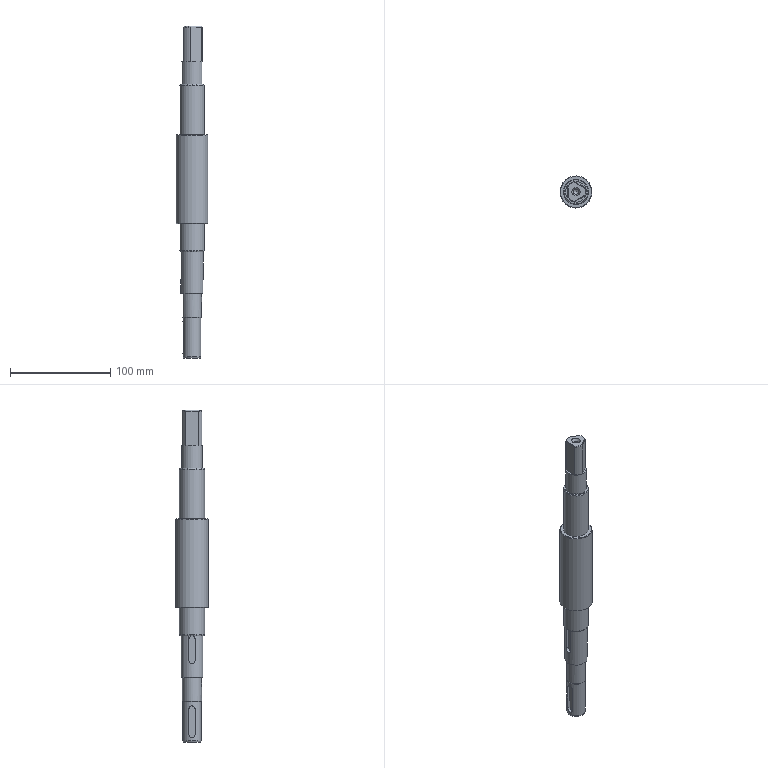NC program | NX | posted with a generic post | part box 32 x 32 x 331.3 mm
Lines 26 to 959 of 3379:
(ZLEVEL_PROFILE , TOOL : D12)
N44 T12 M6
N46 G54
N48 G17 G0 G90 X2.858 Y-14.112 B0. C0. S3000 M3
N50 G43 Z30. H12
N52 Z3.
N54 G94 G1 X1.878 Y-14.678 Z2.97 F1000.
N56 X1.831 Y-14.699 Z2.969
N58 X1.427 Y-14.934 Z2.957
N60 X1.001 Y-15.192 Z2.944
N62 X0.023 Y-15.693 Z2.915
N64 X-1.127 Y-16.017 Z2.884
N66 X-2.318 Y-16.109 Z2.852
N68 X-2.915 Y-16.036 Z2.837
N70 X-3.072 Y-16.017 Z2.833
N72 X-5.029 Y-15.657 Z2.78
N74 X-7.08 Y-14.962 Z2.724
N76 X-7.355 Y-14.847 Z2.716
N78 X-8.788 Y-14.141 Z2.674
N80 X-8.843 Y-14.118 Z2.672
N82 X-9.05 Y-14.001 Z2.666
N84 X-10.687 Y-12.925 Z2.615
N86 X-10.869 Y-12.784 Z2.609
N88 X-11.079 Y-12.619 Z2.602
N90 X-12.428 Y-11.41 Z2.555
N92 X-12.651 Y-11.181 Z2.546
N94 X-13.853 Y-9.785 Z2.498
N96 X-14.227 Y-9.302 Z2.482
N98 X-14.846 Y-8.002 Z2.444
N100 X-15.15 Y-6.595 Z2.407
N102 Y-5.985 Z2.391
N104 Y5.985 Z2.077
N106 X-15.152 Y6.593 Z2.061
N108 X-14.802 Y8.127 Z2.02
N110 X-14.077 Y9.524 Z1.979
N112 X-13.683 Y9.987 Z1.963
N114 X-12.756 Y11.07 Z1.926
N116 X-12.545 Y11.293 Z1.917
N118 X-11.116 Y12.59 Z1.867
N120 X-10.866 Y12.786 Z1.859
N122 X-9.251 Y13.882 Z1.808
N124 X-8.895 Y14.089 Z1.797
N126 X-7.378 Y14.834 Z1.752
N128 X-7.006 Y14.992 Z1.742
N130 X-5.308 Y15.565 Z1.695
N132 X-4.231 Y15.83 Z1.666
N134 X-3.137 Y16.009 Z1.637
N136 X-2.539 Y16.103 Z1.621
N138 X-1.05 Y16.006 Z1.582
N140 X0.371 Y15.552 Z1.543
N142 X0.894 Y15.246 Z1.527
N144 X10.315 Y9.803 Z1.242
N146 X11.822 Y8.929 Z1.197
N148 X12.828 Y8.019 Z1.161
N150 X13.61 Y6.909 Z1.125
N152 X13.848 Y6.352 Z1.11
N154 X14.242 Y5.407 Z1.083
N156 X14.801 Y3.449 Z1.029
N158 X14.965 Y2.438 Z1.003
N160 X15.109 Y1.428 Z0.976
N162 X15.148 Y-0.892 Z0.915
N164 X15.037 Y-1.907 Z0.888
N166 X14.905 Y-2.923 Z0.862
N168 X14.326 Y-5.155 Z0.801
N170 X13.948 Y-6.106 Z0.774
N172 X13.724 Y-6.681 Z0.758
N174 X12.892 Y-7.93 Z0.719
N176 X11.79 Y-8.95 Z0.68
N178 X11.258 Y-9.262 Z0.663
N180 X1.878 Y-14.678 Z0.38
N182 X1.831 Y-14.699 Z0.378
N184 X1.427 Y-14.934 Z0.366
N186 X1.001 Y-15.192 Z0.353
N188 X0.023 Y-15.693 Z0.324
N190 X-1.127 Y-16.017 Z0.293
N192 X-2.318 Y-16.109 Z0.262
N194 X-2.915 Y-16.036 Z0.246
N196 X-3.072 Y-16.017 Z0.242
N198 X-5.029 Y-15.657 Z0.19
N200 X-7.08 Y-14.962 Z0.133
N202 X-7.355 Y-14.847 Z0.125
N204 X-8.788 Y-14.141 Z0.084
N206 X-8.843 Y-14.118 Z0.082
N208 X-9.05 Y-14.001 Z0.076
N210 X-10.687 Y-12.925 Z0.024
N212 X-10.869 Y-12.784 Z0.018
N214 X-11.079 Y-12.619 Z0.011
N216 X-12.428 Y-11.41 Z-0.036
N218 X-12.651 Y-11.181 Z-0.044
N220 X-13.853 Y-9.785 Z-0.093
N222 X-14.227 Y-9.302 Z-0.109
N224 X-14.846 Y-8.002 Z-0.146
N226 X-15.15 Y-6.595 Z-0.184
N228 Y-5.985 Z-0.2
N230 Y5.985 F2200.
N232 G2 X-13.683 Y9.987 R6.15
N234 G1 X-12.756 Y11.07
N236 X-12.545 Y11.293
N238 X-11.116 Y12.59
N240 X-10.866 Y12.786
N242 X-9.251 Y13.882
N244 X-8.895 Y14.089
N246 X-7.378 Y14.834
N248 X-7.006 Y14.992
N250 X-5.308 Y15.565
N252 G2 X-3.137 Y16.009 R28.099
N254 X0.894 Y15.246 R6.1
N256 G1 X10.315 Y9.803
N258 X11.297 Y9.233
N260 G2 X13.848 Y6.352 R6.106
N262 X14.965 Y2.438 R17.455
N264 X15.037 Y-1.907 R17.363
N266 X13.948 Y-6.106 R17.465
N268 X11.258 Y-9.262 R6.316
N270 G1 X1.878 Y-14.678
N272 X1.831 Y-14.699
N274 X1.427 Y-14.934
N276 G2 X0.558 Y-15.419 R14.006
N278 X-2.915 Y-16.036 R6.022
N280 G1 X-3.072 Y-16.017
N282 X-5.029 Y-15.657
N284 X-7.08 Y-14.962
N286 X-7.355 Y-14.847
N288 X-8.788 Y-14.141
N290 X-8.843 Y-14.118
N292 X-9.05 Y-14.001
N294 X-10.687 Y-12.925
N296 X-10.869 Y-12.784
N298 X-11.079 Y-12.619
N300 X-12.428 Y-11.41
N302 X-12.651 Y-11.181
N304 X-13.853 Y-9.785
N306 G2 X-15.15 Y-5.985 R6.204
N308 G1 Y5.473 Z-0.4
N310 Y5.985
N312 G2 X-13.683 Y9.987 R6.15
N314 G1 X-12.756 Y11.07
N316 X-12.545 Y11.293
N318 X-11.116 Y12.59
N320 X-10.866 Y12.786
N322 X-9.251 Y13.882
N324 X-8.895 Y14.089
N326 X-7.379 Y14.834
N328 X-7.006 Y14.992
N330 X-5.308 Y15.565
N332 G2 X-3.137 Y16.009 R28.031
N334 X0.894 Y15.246 R6.1
N336 G1 X10.315 Y9.803
N338 X11.298 Y9.233
N340 G2 X13.848 Y6.352 R6.106
N342 X14.965 Y2.438 R17.431
N344 X15.037 Y-1.907 R17.343
N346 X13.948 Y-6.106 R17.439
N348 X11.258 Y-9.262 R6.318
N350 G1 X1.878 Y-14.678
N352 X1.831 Y-14.699
N354 X1.427 Y-14.934
N356 G2 X0.558 Y-15.419 R14.006
N358 X-2.915 Y-16.036 R6.022
N360 G1 X-3.072 Y-16.017
N362 X-5.028 Y-15.657
N364 X-7.08 Y-14.962
N366 X-7.355 Y-14.847
N368 X-8.843 Y-14.118
N370 X-9.05 Y-14.001
N372 X-10.685 Y-12.926
N374 X-10.869 Y-12.784
N376 X-11.079 Y-12.619
N378 X-12.428 Y-11.41
N380 X-12.651 Y-11.181
N382 X-13.853 Y-9.785
N384 G2 X-15.15 Y-5.985 R6.204
N386 G1 Y5.473 Z-0.6
N388 Y5.985
N390 G2 X-13.683 Y9.987 R6.15
N392 G1 X-12.756 Y11.07
N394 X-12.545 Y11.293
N396 X-11.116 Y12.59
N398 X-10.866 Y12.786
N400 X-9.251 Y13.882
N402 X-8.895 Y14.089
N404 X-7.379 Y14.834
N406 X-7.006 Y14.992
N408 X-5.308 Y15.565
N410 G2 X-3.137 Y16.009 R27.539
N412 X0.894 Y15.246 R6.106
N414 G1 X10.315 Y9.803
N416 X11.298 Y9.233
N418 G2 X13.848 Y6.352 R6.105
N420 X14.965 Y2.438 R17.407
N422 X15.037 Y-1.907 R17.323
N424 X13.948 Y-6.106 R17.414
N426 X11.258 Y-9.262 R6.319
N428 G1 X1.878 Y-14.678
N430 X1.831 Y-14.699
N432 X1.427 Y-14.934
N434 G2 X0.558 Y-15.419 R14.006
N436 X-2.915 Y-16.036 R6.022
N438 G1 X-3.072 Y-16.017
N440 X-5.028 Y-15.657
N442 X-7.08 Y-14.962
N444 X-7.355 Y-14.847
N446 X-8.843 Y-14.118
N448 X-9.05 Y-14.001
N450 X-10.683 Y-12.927
N452 X-10.91 Y-12.752
N454 G2 X-13.899 Y-9.72 R17.164
N456 X-15.15 Y-5.985 R6.133
N458 G1 Y5.473 Z-0.8
N460 Y5.985
N462 G2 X-13.683 Y9.987 R6.15
N464 G1 X-12.756 Y11.07
N466 X-12.545 Y11.293
N468 X-11.116 Y12.59
N470 X-10.866 Y12.786
N472 X-9.251 Y13.882
N474 X-8.895 Y14.089
N476 X-7.379 Y14.834
N478 X-7.006 Y14.992
N480 X-5.308 Y15.565
N482 G2 X-3.136 Y16.009 R27.473
N484 X0.894 Y15.246 R6.107
N486 G1 X10.315 Y9.803
N488 X11.298 Y9.233
N490 G2 X13.848 Y6.352 R6.105
N492 X14.965 Y2.438 R17.384
N494 X15.037 Y-1.907 R17.303
N496 X13.948 Y-6.106 R17.388
N498 X11.258 Y-9.262 R6.321
N500 G1 X1.878 Y-14.678
N502 X1.832 Y-14.699
N504 X1.427 Y-14.934
N506 G2 X0.558 Y-15.419 R14.006
N508 X-2.915 Y-16.036 R6.022
N510 G1 X-3.072 Y-16.017
N512 X-5.028 Y-15.657
N514 X-7.08 Y-14.962
N516 X-7.355 Y-14.847
N518 X-8.843 Y-14.118
N520 X-9.05 Y-14.001
N522 X-10.681 Y-12.929
N524 X-11.036 Y-12.655
N526 G2 X-13.899 Y-9.72 R17.262
N528 X-15.15 Y-5.985 R6.133
N530 G1 Y5.473 Z-1.
N532 Y5.985
N534 G2 X-13.91 Y9.704 R6.189
N536 X-2.955 Y16.031 R16.15
N538 X0.894 Y15.246 R6.198
N540 G1 X11.258 Y9.262
N542 G2 X13.852 Y6.345 R6.172
N544 X13.852 Y-6.345 R16.15
N546 X11.258 Y-9.262 R6.172
N548 G1 X0.954 Y-15.211
N550 G2 X-2.955 Y-16.031 R6.301
N552 X-13.91 Y-9.704 R16.15
N554 X-15.15 Y-5.985 R6.189
N556 G1 Y5.473 Z-1.2
N558 Y6.
N560 G2 X-13.92 Y9.69 R6.15
N562 X-2.932 Y16.034 R16.15
N564 X0.879 Y15.254 R6.15
N566 G1 X11.271 Y9.254
N568 G2 X13.852 Y6.344 R6.15
N570 X13.852 Y-6.344 R16.15
N572 X11.271 Y-9.254 R6.15
N574 G1 X0.879 Y-15.254
N576 G2 X-2.932 Y-16.034 R6.15
N578 X-13.92 Y-9.69 R16.15
N580 X-15.15 Y-5.985 R6.15
N582 G1 Y5.473 Z-1.4
N584 Y6.
N586 G2 X-13.92 Y9.69 R6.15
N588 X-2.932 Y16.034 R16.15
N590 X0.879 Y15.254 R6.15
N592 G1 X11.271 Y9.254
N594 G2 X13.852 Y6.344 R6.15
N596 X13.852 Y-6.344 R16.15
N598 X11.271 Y-9.254 R6.15
N600 G1 X0.879 Y-15.254
N602 G2 X-2.932 Y-16.034 R6.15
N604 X-13.92 Y-9.69 R16.15
N606 X-15.15 Y-5.985 R6.15
N608 G1 Y5.473 Z-1.6
N610 Y6.
N612 G2 X-13.92 Y9.69 R6.15
N614 X-2.932 Y16.034 R16.15
N616 X0.879 Y15.254 R6.15
N618 G1 X11.271 Y9.254
N620 G2 X13.852 Y6.344 R6.15
N622 X13.852 Y-6.344 R16.15
N624 X11.271 Y-9.254 R6.15
N626 G1 X0.879 Y-15.254
N628 G2 X-2.932 Y-16.034 R6.15
N630 X-13.92 Y-9.69 R16.15
N632 X-15.15 Y-5.985 R6.15
N634 G1 Y5.473 Z-1.8
N636 Y6.
N638 G2 X-13.92 Y9.69 R6.15
N640 X-2.932 Y16.034 R16.15
N642 X0.879 Y15.254 R6.15
N644 G1 X11.271 Y9.254
N646 G2 X13.852 Y6.344 R6.15
N648 X13.852 Y-6.344 R16.15
N650 X11.271 Y-9.254 R6.15
N652 G1 X0.879 Y-15.254
N654 G2 X-2.932 Y-16.034 R6.15
N656 X-13.92 Y-9.69 R16.15
N658 X-15.15 Y-5.985 R6.15
N660 G1 Y5.473 Z-2.
N662 Y6.
N664 G2 X-13.92 Y9.69 R6.15
N666 X-2.932 Y16.034 R16.15
N668 X0.879 Y15.254 R6.15
N670 G1 X11.271 Y9.254
N672 G2 X13.852 Y6.344 R6.15
N674 X13.852 Y-6.344 R16.15
N676 X11.271 Y-9.254 R6.15
N678 G1 X0.879 Y-15.254
N680 G2 X-2.932 Y-16.034 R6.15
N682 X-13.92 Y-9.69 R16.15
N684 X-15.15 Y-5.985 R6.15
N686 G1 Y5.473 Z-2.2
N688 Y6.
N690 G2 X-13.92 Y9.69 R6.15
N692 X-2.932 Y16.034 R16.15
N694 X0.879 Y15.254 R6.15
N696 G1 X11.271 Y9.254
N698 G2 X13.852 Y6.344 R6.15
N700 X13.852 Y-6.344 R16.15
N702 X11.271 Y-9.254 R6.15
N704 G1 X0.879 Y-15.254
N706 G2 X-2.932 Y-16.034 R6.15
N708 X-13.92 Y-9.69 R16.15
N710 X-15.15 Y-5.985 R6.15
N712 G1 Y5.473 Z-2.4
N714 Y6.
N716 G2 X-13.92 Y9.69 R6.15
N718 X-2.932 Y16.034 R16.15
N720 X0.879 Y15.254 R6.15
N722 G1 X11.271 Y9.254
N724 G2 X13.852 Y6.344 R6.15
N726 X13.852 Y-6.344 R16.15
N728 X11.271 Y-9.254 R6.15
N730 G1 X0.879 Y-15.254
N732 G2 X-2.932 Y-16.034 R6.15
N734 X-13.92 Y-9.69 R16.15
N736 X-15.15 Y-5.985 R6.15
N738 G1 Y5.473 Z-2.6
N740 Y6.
N742 G2 X-13.92 Y9.69 R6.15
N744 X-2.932 Y16.034 R16.15
N746 X0.879 Y15.254 R6.15
N748 G1 X11.271 Y9.254
N750 G2 X13.852 Y6.344 R6.15
N752 X13.852 Y-6.344 R16.15
N754 X11.271 Y-9.254 R6.15
N756 G1 X0.879 Y-15.254
N758 G2 X-2.932 Y-16.034 R6.15
N760 X-13.92 Y-9.69 R16.15
N762 X-15.15 Y-5.985 R6.15
N764 G1 Y5.473 Z-2.8
N766 Y6.
N768 G2 X-13.92 Y9.69 R6.15
N770 X-2.932 Y16.034 R16.15
N772 X0.879 Y15.254 R6.15
N774 G1 X11.271 Y9.254
N776 G2 X13.852 Y6.344 R6.15
N778 X13.852 Y-6.344 R16.15
N780 X11.271 Y-9.254 R6.15
N782 G1 X0.879 Y-15.254
N784 G2 X-2.932 Y-16.034 R6.15
N786 X-13.92 Y-9.69 R16.15
N788 X-15.15 Y-5.985 R6.15
N790 G1 Y5.473 Z-3.
N792 Y6.
N794 G2 X-13.92 Y9.69 R6.15
N796 X-2.932 Y16.034 R16.15
N798 X0.879 Y15.254 R6.15
N800 G1 X11.271 Y9.254
N802 G2 X13.852 Y6.344 R6.15
N804 X13.852 Y-6.344 R16.15
N806 X11.271 Y-9.254 R6.15
N808 G1 X0.879 Y-15.254
N810 G2 X-2.932 Y-16.034 R6.15
N812 X-13.92 Y-9.69 R16.15
N814 X-15.15 Y-5.985 R6.15
N816 G1 Y5.473 Z-3.2
N818 Y6.
N820 G2 X-13.92 Y9.69 R6.15
N822 X-2.932 Y16.034 R16.15
N824 X0.879 Y15.254 R6.15
N826 G1 X11.271 Y9.254
N828 G2 X13.852 Y6.344 R6.15
N830 X13.852 Y-6.344 R16.15
N832 X11.271 Y-9.254 R6.15
N834 G1 X0.879 Y-15.254
N836 G2 X-2.932 Y-16.034 R6.15
N838 X-13.92 Y-9.69 R16.15
N840 X-15.15 Y-5.985 R6.15
N842 G1 Y5.473 Z-3.4
N844 Y6.
N846 G2 X-13.92 Y9.69 R6.15
N848 X-2.932 Y16.034 R16.15
N850 X0.879 Y15.254 R6.15
N852 G1 X11.271 Y9.254
N854 G2 X13.852 Y6.344 R6.15
N856 X13.852 Y-6.344 R16.15
N858 X11.271 Y-9.254 R6.15
N860 G1 X0.879 Y-15.254
N862 G2 X-2.932 Y-16.034 R6.15
N864 X-13.92 Y-9.69 R16.15
N866 X-15.15 Y-5.985 R6.15
N868 G1 Y5.473 Z-3.6
N870 Y6.
N872 G2 X-13.92 Y9.69 R6.15
N874 X-2.932 Y16.034 R16.15
N876 X0.879 Y15.254 R6.15
N878 G1 X11.271 Y9.254
N880 G2 X13.852 Y6.344 R6.15
N882 X13.852 Y-6.344 R16.15
N884 X11.271 Y-9.254 R6.15
N886 G1 X0.879 Y-15.254
N888 G2 X-2.932 Y-16.034 R6.15
N890 X-13.92 Y-9.69 R16.15
N892 X-15.15 Y-5.985 R6.15
N894 G1 Y5.473 Z-3.8
N896 Y6.
N898 G2 X-13.92 Y9.69 R6.15
N900 X-2.932 Y16.034 R16.15
N902 X0.879 Y15.254 R6.15
N904 G1 X11.271 Y9.254
N906 G2 X13.852 Y6.344 R6.15
N908 X13.852 Y-6.344 R16.15
N910 X11.271 Y-9.254 R6.15
N912 G1 X0.879 Y-15.254
N914 G2 X-2.932 Y-16.034 R6.15
N916 X-13.92 Y-9.69 R16.15
N918 X-15.15 Y-5.985 R6.15
N920 G1 Y5.473 Z-4.
N922 Y6.
N924 G2 X-13.92 Y9.69 R6.15
N926 X-2.932 Y16.034 R16.15
N928 X0.879 Y15.254 R6.15
N930 G1 X11.271 Y9.254
N932 G2 X13.852 Y6.344 R6.15
N934 X13.852 Y-6.344 R16.15
N936 X11.271 Y-9.254 R6.15
N938 G1 X0.879 Y-15.254
N940 G2 X-2.932 Y-16.034 R6.15
N942 X-13.92 Y-9.69 R16.15
N944 X-15.15 Y-5.985 R6.15
N946 G1 Y5.473 Z-4.2
N948 Y6.
N950 G2 X-13.92 Y9.69 R6.15
N952 X-2.932 Y16.034 R16.15
N954 X0.879 Y15.254 R6.15
N956 G1 X11.271 Y9.254
N958 G2 X13.852 Y6.344 R6.15
N960 X13.852 Y-6.344 R16.15
N962 X11.271 Y-9.254 R6.15
N964 G1 X0.879 Y-15.254
N966 G2 X-2.932 Y-16.034 R6.15
N968 X-13.92 Y-9.69 R16.15
N970 X-15.15 Y-5.985 R6.15
N972 G1 Y5.473 Z-4.4
N974 Y6.
N976 G2 X-13.92 Y9.69 R6.15
N978 X-2.932 Y16.034 R16.15
N980 X0.879 Y15.254 R6.15
N982 G1 X11.271 Y9.254
N984 G2 X13.852 Y6.344 R6.15
N986 X13.852 Y-6.344 R16.15
N988 X11.271 Y-9.254 R6.15
N990 G1 X0.879 Y-15.254
N992 G2 X-2.932 Y-16.034 R6.15
N994 X-13.92 Y-9.69 R16.15
N996 X-15.15 Y-5.985 R6.15
N998 G1 Y5.473 Z-4.6
N1000 Y6.
N1002 G2 X-13.92 Y9.69 R6.15
N1004 X-2.932 Y16.034 R16.15
N1006 X0.879 Y15.254 R6.15
N1008 G1 X11.271 Y9.254
N1010 G2 X13.852 Y6.344 R6.15
N1012 X13.852 Y-6.344 R16.15
N1014 X11.271 Y-9.254 R6.15
N1016 G1 X0.879 Y-15.254
N1018 G2 X-2.932 Y-16.034 R6.15
N1020 X-13.92 Y-9.69 R16.15
N1022 X-15.15 Y-5.985 R6.15
N1024 G1 Y5.473 Z-4.8
N1026 Y6.
N1028 G2 X-13.92 Y9.69 R6.15
N1030 X-2.932 Y16.034 R16.15
N1032 X0.879 Y15.254 R6.15
N1034 G1 X11.271 Y9.254
N1036 G2 X13.852 Y6.344 R6.15
N1038 X13.852 Y-6.344 R16.15
N1040 X11.271 Y-9.254 R6.15
N1042 G1 X0.879 Y-15.254
N1044 G2 X-2.932 Y-16.034 R6.15
N1046 X-13.92 Y-9.69 R16.15
N1048 X-15.15 Y-5.985 R6.15
N1050 G1 Y5.473 Z-5.
N1052 Y6.
N1054 G2 X-13.92 Y9.69 R6.15
N1056 X-2.932 Y16.034 R16.15
N1058 X0.879 Y15.254 R6.15
N1060 G1 X11.271 Y9.254
N1062 G2 X13.852 Y6.344 R6.15
N1064 X13.852 Y-6.344 R16.15
N1066 X11.271 Y-9.254 R6.15
N1068 G1 X0.879 Y-15.254
N1070 G2 X-2.932 Y-16.034 R6.15
N1072 X-13.92 Y-9.69 R16.15
N1074 X-15.15 Y-5.985 R6.15
N1076 G1 Y5.473 Z-5.2
N1078 Y6.
N1080 G2 X-13.92 Y9.69 R6.15
N1082 X-2.932 Y16.034 R16.15
N1084 X0.879 Y15.254 R6.15
N1086 G1 X11.271 Y9.254
N1088 G2 X13.852 Y6.344 R6.15
N1090 X13.852 Y-6.344 R16.15
N1092 X11.271 Y-9.254 R6.15
N1094 G1 X0.879 Y-15.254
N1096 G2 X-2.932 Y-16.034 R6.15
N1098 X-13.92 Y-9.69 R16.15
N1100 X-15.15 Y-5.985 R6.15
N1102 G1 Y5.473 Z-5.4
N1104 Y6.
N1106 G2 X-13.92 Y9.69 R6.15
N1108 X-2.932 Y16.034 R16.15
N1110 X0.879 Y15.254 R6.15
N1112 G1 X11.271 Y9.254
N1114 G2 X13.852 Y6.344 R6.15
N1116 X13.852 Y-6.344 R16.15
N1118 X11.271 Y-9.254 R6.15
N1120 G1 X0.879 Y-15.254
N1122 G2 X-2.932 Y-16.034 R6.15
N1124 X-13.92 Y-9.69 R16.15
N1126 X-15.15 Y-5.985 R6.15
N1128 G1 Y5.473 Z-5.6
N1130 Y6.
N1132 G2 X-13.92 Y9.69 R6.15
N1134 X-2.932 Y16.034 R16.15
N1136 X0.879 Y15.254 R6.15
N1138 G1 X11.271 Y9.254
N1140 G2 X13.852 Y6.344 R6.15
N1142 X13.852 Y-6.344 R16.15
N1144 X11.271 Y-9.254 R6.15
N1146 G1 X0.879 Y-15.254
N1148 G2 X-2.932 Y-16.034 R6.15
N1150 X-13.92 Y-9.69 R16.15
N1152 X-15.15 Y-5.985 R6.15
N1154 G1 Y5.473 Z-5.8
N1156 Y6.
N1158 G2 X-13.92 Y9.69 R6.15
N1160 X-2.932 Y16.034 R16.15
N1162 X0.879 Y15.254 R6.15
N1164 G1 X11.271 Y9.254
N1166 G2 X13.852 Y6.344 R6.15
N1168 X13.852 Y-6.344 R16.15
N1170 X11.271 Y-9.254 R6.15
N1172 G1 X0.879 Y-15.254
N1174 G2 X-2.932 Y-16.034 R6.15
N1176 X-13.92 Y-9.69 R16.15
N1178 X-15.15 Y-5.985 R6.15
N1180 G1 Y5.473 Z-6.
N1182 Y6.
N1184 G2 X-13.92 Y9.69 R6.15
N1186 X-2.932 Y16.034 R16.15
N1188 X0.879 Y15.254 R6.15
N1190 G1 X11.271 Y9.254
N1192 G2 X13.852 Y6.344 R6.15
N1194 X13.852 Y-6.344 R16.15
N1196 X11.271 Y-9.254 R6.15
N1198 G1 X0.879 Y-15.254
N1200 G2 X-2.932 Y-16.034 R6.15
N1202 X-13.92 Y-9.69 R16.15
N1204 X-15.15 Y-5.985 R6.15
N1206 G1 Y5.473 Z-6.2
N1208 Y6.
N1210 G2 X-13.92 Y9.69 R6.15
N1212 X-2.932 Y16.034 R16.15
N1214 X0.879 Y15.254 R6.15
N1216 G1 X11.271 Y9.254
N1218 G2 X13.852 Y6.344 R6.15
N1220 X13.852 Y-6.344 R16.15
N1222 X11.271 Y-9.254 R6.15
N1224 G1 X0.879 Y-15.254
N1226 G2 X-2.932 Y-16.034 R6.15
N1228 X-13.92 Y-9.69 R16.15
N1230 X-15.15 Y-5.985 R6.15
N1232 G1 Y5.473 Z-6.4
N1234 Y6.
N1236 G2 X-13.92 Y9.69 R6.15
N1238 X-2.932 Y16.034 R16.15
N1240 X0.879 Y15.254 R6.15
N1242 G1 X11.271 Y9.254
N1244 G2 X13.852 Y6.344 R6.15
N1246 X13.852 Y-6.344 R16.15
N1248 X11.271 Y-9.254 R6.15
N1250 G1 X0.879 Y-15.254
N1252 G2 X-2.932 Y-16.034 R6.15
N1254 X-13.92 Y-9.69 R16.15
N1256 X-15.15 Y-5.985 R6.15
N1258 G1 Y5.473 Z-6.6
N1260 Y6.
N1262 G2 X-13.92 Y9.69 R6.15
N1264 X-2.932 Y16.034 R16.15
N1266 X0.879 Y15.254 R6.15
N1268 G1 X11.271 Y9.254
N1270 G2 X13.852 Y6.344 R6.15
N1272 X13.852 Y-6.344 R16.15
N1274 X11.271 Y-9.254 R6.15
N1276 G1 X0.879 Y-15.254
N1278 G2 X-2.932 Y-16.034 R6.15
N1280 X-13.92 Y-9.69 R16.15
N1282 X-15.15 Y-5.985 R6.15
N1284 G1 Y5.473 Z-6.8
N1286 Y6.
N1288 G2 X-13.92 Y9.69 R6.15
N1290 X-2.932 Y16.034 R16.15
N1292 X0.879 Y15.254 R6.15
N1294 G1 X11.271 Y9.254
N1296 G2 X13.852 Y6.344 R6.15
N1298 X13.852 Y-6.344 R16.15
N1300 X11.271 Y-9.254 R6.15
N1302 G1 X0.879 Y-15.254
N1304 G2 X-2.932 Y-16.034 R6.15
N1306 X-13.92 Y-9.69 R16.15
N1308 X-15.15 Y-5.985 R6.15
N1310 G1 Y5.473 Z-7.
N1312 Y6.
N1314 G2 X-13.92 Y9.69 R6.15
N1316 X-2.932 Y16.034 R16.15
N1318 X0.879 Y15.254 R6.15
N1320 G1 X11.271 Y9.254
N1322 G2 X13.852 Y6.344 R6.15
N1324 X13.852 Y-6.344 R16.15
N1326 X11.271 Y-9.254 R6.15
N1328 G1 X0.879 Y-15.254
N1330 G2 X-2.932 Y-16.034 R6.15
N1332 X-13.92 Y-9.69 R16.15
N1334 X-15.15 Y-5.985 R6.15
N1336 G1 Y5.473 Z-7.2
N1338 Y6.
N1340 G2 X-13.92 Y9.69 R6.15
N1342 X-2.932 Y16.034 R16.15
N1344 X0.879 Y15.254 R6.15
N1346 G1 X11.271 Y9.254
N1348 G2 X13.852 Y6.344 R6.15
N1350 X13.852 Y-6.344 R16.15
N1352 X11.271 Y-9.254 R6.15
N1354 G1 X0.879 Y-15.254
N1356 G2 X-2.932 Y-16.034 R6.15
N1358 X-13.92 Y-9.69 R16.15
N1360 X-15.15 Y-5.985 R6.15
N1362 G1 Y5.473 Z-7.4
N1364 Y6.
N1366 G2 X-13.92 Y9.69 R6.15
N1368 X-2.932 Y16.034 R16.15
N1370 X0.879 Y15.254 R6.15
N1372 G1 X11.271 Y9.254
N1374 G2 X13.852 Y6.344 R6.15
N1376 X13.852 Y-6.344 R16.15
N1378 X11.271 Y-9.254 R6.15
N1380 G1 X0.879 Y-15.254
N1382 G2 X-2.932 Y-16.034 R6.15
N1384 X-13.92 Y-9.69 R16.15
N1386 X-15.15 Y-5.985 R6.15
N1388 G1 Y5.473 Z-7.6
N1390 Y6.
N1392 G2 X-13.92 Y9.69 R6.15
N1394 X-2.932 Y16.034 R16.15
N1396 X0.879 Y15.254 R6.15
N1398 G1 X11.271 Y9.254
N1400 G2 X13.852 Y6.344 R6.15
N1402 X13.852 Y-6.344 R16.15
N1404 X11.271 Y-9.254 R6.15
N1406 G1 X0.879 Y-15.254
N1408 G2 X-2.932 Y-16.034 R6.15
N1410 X-13.92 Y-9.69 R16.15
N1412 X-15.15 Y-5.985 R6.15
N1414 G1 Y5.473 Z-7.8
N1416 Y6.
N1418 G2 X-13.92 Y9.69 R6.15
N1420 X-2.932 Y16.034 R16.15
N1422 X0.879 Y15.254 R6.15
N1424 G1 X11.271 Y9.254
N1426 G2 X13.852 Y6.344 R6.15
N1428 X13.852 Y-6.344 R16.15
N1430 X11.271 Y-9.254 R6.15
N1432 G1 X0.879 Y-15.254
N1434 G2 X-2.932 Y-16.034 R6.15
N1436 X-13.92 Y-9.69 R16.15
N1438 X-15.15 Y-5.985 R6.15
N1440 G1 Y5.473 Z-8.
N1442 Y6.
N1444 G2 X-13.92 Y9.69 R6.15
N1446 X-2.932 Y16.034 R16.15
N1448 X0.879 Y15.254 R6.15
N1450 G1 X11.271 Y9.254
N1452 G2 X13.852 Y6.344 R6.15
N1454 X13.852 Y-6.344 R16.15
N1456 X11.271 Y-9.254 R6.15
N1458 G1 X0.879 Y-15.254
N1460 G2 X-2.932 Y-16.034 R6.15
N1462 X-13.92 Y-9.69 R16.15
N1464 X-15.15 Y-5.985 R6.15
N1466 G1 Y5.473 Z-8.2
N1468 Y6.
N1470 G2 X-13.92 Y9.69 R6.15
N1472 X-2.932 Y16.034 R16.15
N1474 X0.879 Y15.254 R6.15
N1476 G1 X11.271 Y9.254
N1478 G2 X13.852 Y6.344 R6.15
N1480 X13.852 Y-6.344 R16.15
N1482 X11.271 Y-9.254 R6.15
N1484 G1 X0.879 Y-15.254
N1486 G2 X-2.932 Y-16.034 R6.15
N1488 X-13.92 Y-9.69 R16.15
N1490 X-15.15 Y-5.985 R6.15
N1492 G1 Y5.473 Z-8.4
N1494 Y6.
N1496 G2 X-13.92 Y9.69 R6.15
N1498 X-2.932 Y16.034 R16.15
N1500 X0.879 Y15.254 R6.15
N1502 G1 X11.271 Y9.254
N1504 G2 X13.852 Y6.344 R6.15
N1506 X13.852 Y-6.344 R16.15
N1508 X11.271 Y-9.254 R6.15
N1510 G1 X0.879 Y-15.254
N1512 G2 X-2.932 Y-16.034 R6.15
N1514 X-13.92 Y-9.69 R16.15
N1516 X-15.15 Y-5.985 R6.15
N1518 G1 Y5.473 Z-8.6
N1520 Y6.
N1522 G2 X-13.92 Y9.69 R6.15
N1524 X-2.932 Y16.034 R16.15
N1526 X0.879 Y15.254 R6.15
N1528 G1 X11.271 Y9.254
N1530 G2 X13.852 Y6.344 R6.15
N1532 X13.852 Y-6.344 R16.15
N1534 X11.271 Y-9.254 R6.15
N1536 G1 X0.879 Y-15.254
N1538 G2 X-2.932 Y-16.034 R6.15
N1540 X-13.92 Y-9.69 R16.15
N1542 X-15.15 Y-5.985 R6.15
N1544 G1 Y5.473 Z-8.8
N1546 Y6.
N1548 G2 X-13.92 Y9.69 R6.15
N1550 X-2.932 Y16.034 R16.15
N1552 X0.879 Y15.254 R6.15
N1554 G1 X11.271 Y9.254
N1556 G2 X13.852 Y6.344 R6.15
N1558 X13.852 Y-6.344 R16.15
N1560 X11.271 Y-9.254 R6.15
N1562 G1 X0.879 Y-15.254
N1564 G2 X-2.932 Y-16.034 R6.15
N1566 X-13.92 Y-9.69 R16.15
N1568 X-15.15 Y-5.985 R6.15
N1570 G1 Y5.473 Z-9.
N1572 Y6.
N1574 G2 X-13.92 Y9.69 R6.15
N1576 X-2.932 Y16.034 R16.15
N1578 X0.879 Y15.254 R6.15
N1580 G1 X11.271 Y9.254
N1582 G2 X13.852 Y6.344 R6.15
N1584 X13.852 Y-6.344 R16.15
N1586 X11.271 Y-9.254 R6.15
N1588 G1 X0.879 Y-15.254
N1590 G2 X-2.932 Y-16.034 R6.15
N1592 X-13.92 Y-9.69 R16.15
N1594 X-15.15 Y-5.985 R6.15
N1596 G1 Y5.473 Z-9.2
N1598 Y6.
N1600 G2 X-13.92 Y9.69 R6.15
N1602 X-2.932 Y16.034 R16.15
N1604 X0.879 Y15.254 R6.15
N1606 G1 X11.271 Y9.254
N1608 G2 X13.852 Y6.344 R6.15
N1610 X13.852 Y-6.344 R16.15
N1612 X11.271 Y-9.254 R6.15
N1614 G1 X0.879 Y-15.254
N1616 G2 X-2.932 Y-16.034 R6.15
N1618 X-13.92 Y-9.69 R16.15
N1620 X-15.15 Y-5.985 R6.15
N1622 G1 Y5.473 Z-9.4
N1624 Y6.
N1626 G2 X-13.92 Y9.69 R6.15
N1628 X-2.932 Y16.034 R16.15
N1630 X0.879 Y15.254 R6.15
N1632 G1 X11.271 Y9.254
N1634 G2 X13.852 Y6.344 R6.15
N1636 X13.852 Y-6.344 R16.15
N1638 X11.271 Y-9.254 R6.15
N1640 G1 X0.879 Y-15.254
N1642 G2 X-2.932 Y-16.034 R6.15
N1644 X-13.92 Y-9.69 R16.15
N1646 X-15.15 Y-5.985 R6.15
N1648 G1 Y5.473 Z-9.6
N1650 Y6.
N1652 G2 X-13.92 Y9.69 R6.15
N1654 X-2.932 Y16.034 R16.15
N1656 X0.879 Y15.254 R6.15
N1658 G1 X11.271 Y9.254
N1660 G2 X13.852 Y6.344 R6.15
N1662 X13.852 Y-6.344 R16.15
N1664 X11.271 Y-9.254 R6.15
N1666 G1 X0.879 Y-15.254
N1668 G2 X-2.932 Y-16.034 R6.15
N1670 X-13.92 Y-9.69 R16.15
N1672 X-15.15 Y-5.985 R6.15
N1674 G1 Y5.473 Z-9.8
N1676 Y6.
N1678 G2 X-13.92 Y9.69 R6.15
N1680 X-2.932 Y16.034 R16.15
N1682 X0.879 Y15.254 R6.15
N1684 G1 X11.271 Y9.254
N1686 G2 X13.852 Y6.344 R6.15
N1688 X13.852 Y-6.344 R16.15
N1690 X11.271 Y-9.254 R6.15
N1692 G1 X0.879 Y-15.254
N1694 G2 X-2.932 Y-16.034 R6.15
N1696 X-13.92 Y-9.69 R16.15
N1698 X-15.15 Y-5.985 R6.15
N1700 G1 Y5.473 Z-10.
N1702 Y6.
N1704 G2 X-13.92 Y9.69 R6.15
N1706 X-2.932 Y16.034 R16.15
N1708 X0.879 Y15.254 R6.15
N1710 G1 X11.271 Y9.254
N1712 G2 X13.852 Y6.344 R6.15
N1714 X13.852 Y-6.344 R16.15
N1716 X11.271 Y-9.254 R6.15
N1718 G1 X0.879 Y-15.254
N1720 G2 X-2.932 Y-16.034 R6.15
N1722 X-13.92 Y-9.69 R16.15
N1724 X-15.15 Y-5.985 R6.15
N1726 G1 Y5.473 Z-10.2
N1728 Y6.
N1730 G2 X-13.92 Y9.69 R6.15
N1732 X-2.932 Y16.034 R16.15
N1734 X0.879 Y15.254 R6.15
N1736 G1 X11.271 Y9.254
N1738 G2 X13.852 Y6.344 R6.15
N1740 X13.852 Y-6.344 R16.15
N1742 X11.271 Y-9.254 R6.15
N1744 G1 X0.879 Y-15.254
N1746 G2 X-2.932 Y-16.034 R6.15
N1748 X-13.92 Y-9.69 R16.15
N1750 X-15.15 Y-5.985 R6.15
N1752 G1 Y5.473 Z-10.4
N1754 Y6.
N1756 G2 X-13.92 Y9.69 R6.15
N1758 X-2.932 Y16.034 R16.15
N1760 X0.879 Y15.254 R6.15
N1762 G1 X11.271 Y9.254
N1764 G2 X13.852 Y6.344 R6.15
N1766 X13.852 Y-6.344 R16.15
N1768 X11.271 Y-9.254 R6.15
N1770 G1 X0.879 Y-15.254
N1772 G2 X-2.932 Y-16.034 R6.15
N1774 X-13.92 Y-9.69 R16.15
N1776 X-15.15 Y-5.985 R6.15
N1778 G1 Y5.473 Z-10.6
N1780 Y6.
N1782 G2 X-13.92 Y9.69 R6.15
N1784 X-2.932 Y16.034 R16.15
N1786 X0.879 Y15.254 R6.15
N1788 G1 X11.271 Y9.254
N1790 G2 X13.852 Y6.344 R6.15
N1792 X13.852 Y-6.344 R16.15
N1794 X11.271 Y-9.254 R6.15
N1796 G1 X0.879 Y-15.254
N1798 G2 X-2.932 Y-16.034 R6.15
N1800 X-13.92 Y-9.69 R16.15
N1802 X-15.15 Y-5.985 R6.15
N1804 G1 Y5.473 Z-10.8
N1806 Y6.
N1808 G2 X-13.92 Y9.69 R6.15
N1810 X-2.932 Y16.034 R16.15
N1812 X0.879 Y15.254 R6.15
N1814 G1 X11.271 Y9.254
N1816 G2 X13.852 Y6.344 R6.15
N1818 X13.852 Y-6.344 R16.15
N1820 X11.271 Y-9.254 R6.15
N1822 G1 X0.879 Y-15.254
N1824 G2 X-2.932 Y-16.034 R6.15
N1826 X-13.92 Y-9.69 R16.15
N1828 X-15.15 Y-5.985 R6.15
N1830 G1 Y5.473 Z-11.
N1832 Y6.
N1834 G2 X-13.92 Y9.69 R6.15
N1836 X-2.932 Y16.034 R16.15
N1838 X0.879 Y15.254 R6.15
N1840 G1 X11.271 Y9.254
N1842 G2 X13.852 Y6.344 R6.15
N1844 X13.852 Y-6.344 R16.15
N1846 X11.271 Y-9.254 R6.15
N1848 G1 X0.879 Y-15.254
N1850 G2 X-2.932 Y-16.034 R6.15
N1852 X-13.92 Y-9.69 R16.15
N1854 X-15.15 Y-5.985 R6.15
N1856 G1 Y5.473 Z-11.2
N1858 Y6.
N1860 G2 X-13.92 Y9.69 R6.15
N1862 X-2.932 Y16.034 R16.15
N1864 X0.879 Y15.254 R6.15
N1866 G1 X11.271 Y9.254
N1868 G2 X13.852 Y6.344 R6.15
N1870 X13.852 Y-6.344 R16.15
N1872 X11.271 Y-9.254 R6.15
N1874 G1 X0.879 Y-15.254
N1876 G2 X-2.932 Y-16.034 R6.15
N1878 X-13.92 Y-9.69 R16.15
N1880 X-15.15 Y-5.985 R6.15
N1882 G1 Y5.473 Z-11.4
N1884 Y6.
N1886 G2 X-13.92 Y9.69 R6.15
N1888 X-2.932 Y16.034 R16.15
N1890 X0.879 Y15.254 R6.15
N1892 G1 X11.271 Y9.254
N1894 G2 X13.852 Y6.344 R6.15
N1896 X13.852 Y-6.344 R16.15
N1898 X11.271 Y-9.254 R6.15
N1900 G1 X0.879 Y-15.254
N1902 G2 X-2.932 Y-16.034 R6.15
N1904 X-13.92 Y-9.69 R16.15